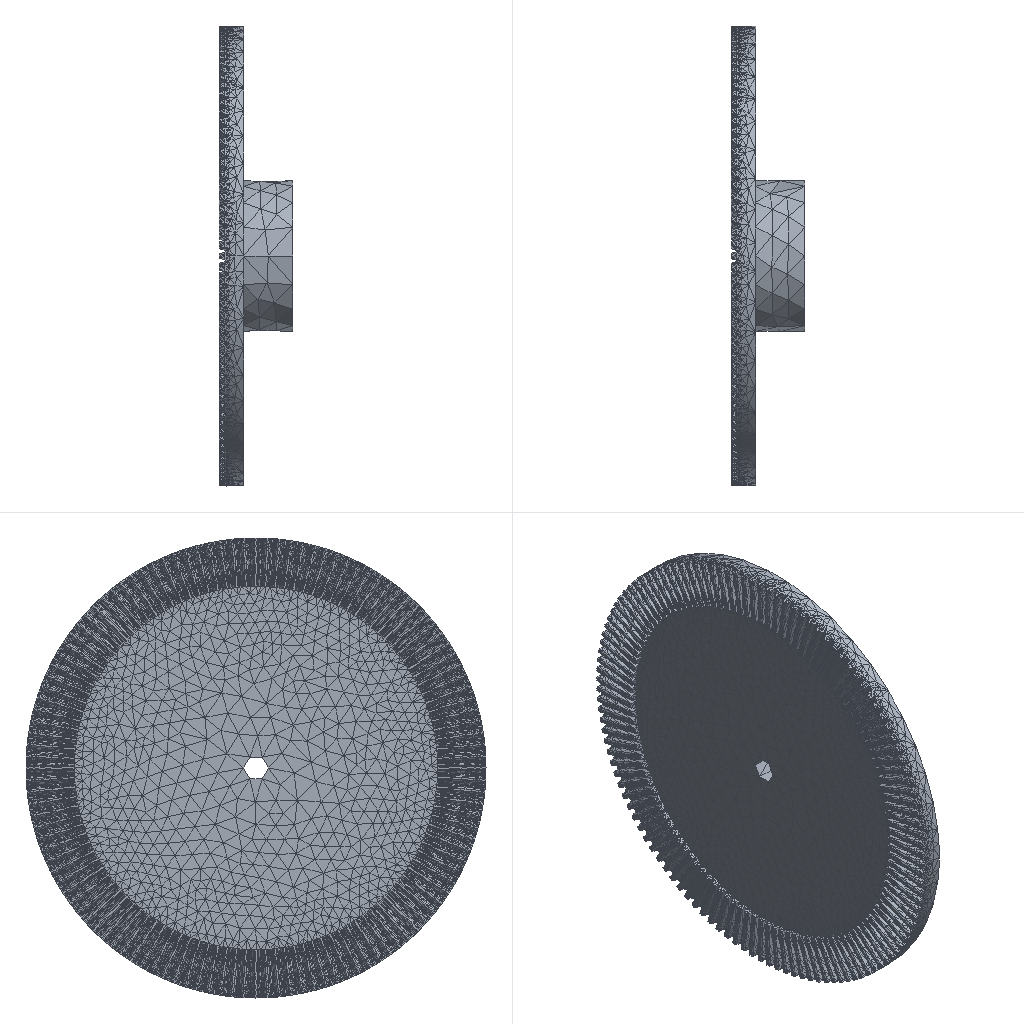Simulation study | ansys workbench
Set-up summary:
category,name,step,type,value,unit,region
solver,ansys_workbench
units,mm-N-s-tonne (MPa),,stated,"/units,MPA"
analysis,LS1,,modal,method=lanb; n_modes=6
load_step,LS1,LS1,modal
mesh,nodes,,,62313
mesh,elements,,,32535
element_type,SOLID187,,,32535
material,45?,,E,200000,tonne s^-2 mm^-1
material,45?,,nu,0.3
material,45?,,density,7.85e-09,tonne mm^-3
material,45?,,conductivity,60.5,tonne mm s^-3 C^-1
material,45?,,specific_heat,4.34e+08,mm^2 s^-2 C^-1
material,45?,,cte,1.2e-05,C^-1
material,45?,,permeability,10000
material,45?,,resistivity,0.00017,ohm mm
bc,Fixed Supports,model,fixed,[dofs=ALL],,_FIXEDSU
named_set,_FIXEDSU,,node,68
Ansys APDL input file, long lists of numbers shortened:
/batch
/config,noeldb,1     ! force off writing results to database
*get,_wallstrt,active,,time,wall
! ANSYS input file written by Workbench version 2022 R1
! File used for geometry attach:
/title,wbnew--__ (B5)
! ****** Begin Custom Load Command Snippet ******
/COM, ACT Extensions:
/COM,     LSDYNA, 2021.1
/COM,
! ****** End   Custom Load Command Snippet ******
*DIM,_wb_ProjectScratch_dir,string,248
_wb_ProjectScratch_dir(1) = ''
*DIM,_wb_SolverFiles_dir,string,248
_wb_SolverFiles_dir(1) = ''
*DIM,_wb_userfiles_dir,string,248
_wb_userfiles_dir(1) = ''
/com,--- Data in consistent NMM units. See Solving Units in the help system for more information.
/units,MPA
/nopr
/wb,file,start              !  signify a WB generated input file
/prep7
! Turn off shape checking because checks already performed inside WB mesher.
! See help system for more information.
SHPP,OFF,,NOWARN
/nolist
etcon,set             ! allow ANSYS to choose best KEYOP's for 180x elements, resets any applicable keyopt to MAPDL defaults
/com,*********** Nodes for the whole assembly ***********
nblock,3,,68544
(1i9,3e20.9e3)
        1    -1.600000000E+01     2.450000000E+01     0.000000000E+00
! (62312 more lines like these left out)
-1
/wb,elem,start            !  set before creation of elements
/com,*********** Elements for Body 1 "60-FreeParts|__-__1" ***********
et,1,187
eblock,19,solid,,32535
(19i9)
        1        1        1        1        0        0        0        0       10        0        1     6731    10302     6958     7188    51539    53095    51534    51537
! (65069 more lines like these left out)
-1
/wb,elem,end               !  done creating elements
/com,*********** Send User Defined Coordinate System(s) ***********
csys,0
toffst,273.15,  ! Temperature offset from absolute zero
/com,*********** Set Reference Temperature ***********
tref,22.
/wb,mat,start              !  starting to send materials
/com,*********** Send Materials ***********
Temperature = 'TEMP' ! Temperature
MP,DENS,1,7.85e-09,	! tonne mm^-3
MP,ALPX,1,1.2e-05,	! C^-1
MP,C,1,434000000,	! mm^2 s^-2 C^-1
MP,KXX,1,60.5,	! tonne mm s^-3 C^-1
MP,RSVX,1,0.00017,	! ohm mm
MP,EX,1,200000,	! tonne s^-2 mm^-1
MP,NUXY,1,0.3,
MP,MURX,1,10000,
/wb,mat,end                !  done sending materials
!************************* Model Summary ********************
!60-FreeParts|__-__1,	45钢,	matid,	1
!************************* End Model Summary ********************
! get the diagonal of the bounding box. Needed later for other things
*get,_xmin,node,,mnloc,x
*get,_ymin,node,,mnloc,y
*get,_zmin,node,,mnloc,z
*get,_xmax,node,,mxloc,x
*get,_ymax,node,,mxloc,y
*get,_zmax,node,,mxloc,z
_ASMDIAG=(_xmax-_xmin)*(_xmax-_xmin)+(_ymax-_ymin)*(_ymax-_ymin)+(_zmax-_zmin)*(_zmax-_zmin)
_ASMDIAG=SQRT(_ASMDIAG)
/wb,contact,start          !  starting to send contact
/wb,contact,end            !  done creating contacts
/golist
/wb,load,start             !  starting to send loads
/com,*********** Fixed Supports ***********
CMBLOCK,_FIXEDSU,NODE,       68
(8i10)
       407       408       409       410       411       412       413       414
! (8 more lines like these left out)
cmsel,s,_FIXEDSU
d,all,all
nsel,all
/gst,on,on
fini
*get,_numnode,node,0,count
*get,_numelem,elem,0,count
*get, _MAXELEMNUM, elem, 0, NUM, MAX
*get, _MAXNODENUM, node, 0, NUM, MAX
*get, _MAXELEMTYPE, etyp, 0, NUM, MAX
*get, _MAXREALCONST, real, 0, NUM, MAX
/go
/wb,load,end               !  done creating loads
/com,--- Number of total nodes = %_numnode%
/com,--- Number of contact elements = 0
/com,--- Number of spring elements = 0
/com,--- Number of bearing elements = 0
/com,--- Number of solid elements = 32535
/com,--- Number of condensed parts = 0
/com,--- Number of total elements = %_numelem%
*get,_wallbsol,active,,time,wall
/solu
antype,2                   ! modal analysis
_thickRatio=  1     ! Ratio of thick parts in the model
modopt,lanb,6
outres,erase
outres,all,none
outres,nsol,all
outres,etmp,all
mxpand                    ! default expand in case of complex solution
dmpopt,esav,no
dmpopt,emat,no
dmpopt,full,no
! *********** WB SOLVE COMMAND ***********
! check interactive state
*get,ANSINTER_,active,,int
*if,ANSINTER_,ne,0,then
/eof
*endif
solve
/com *************** Write FE CONNECTORS *********
CEWRITE,file,ce,,INTE
*get,_nmodalsolproc,active,0,numcpu
fini
/nopr
*get,_numnode,node,0,count
*get,_numelem,elem,0,count
*get, _MAXELEMNUM, elem, 0, NUM, MAX
*get, _MAXNODENUM, node, 0, NUM, MAX,,,INTERNAL
*get, _MAXELEMTYPE, etyp, 0, NUM, MAX
*get, _MAXREALCONST, real, 0, NUM, MAX
/gopr
*get,_wallasol,active,,time,wall
/post1
/nopr
*dim,_direction,CHAR,6,1
_direction(1) = 'X'
_direction(2) = 'Y'
_direction(3) = 'Z'
_direction(4) = 'ROTX'
_direction(5) = 'ROTY'
_direction(6) = 'ROTZ'
*get,_lastLS,active,0,set,LSTP
*get,_beginset,active,0,set,nset,first,_lastLS
*get,_endset,active,0,set,nset,last,_lastLS
_nummodes = 0
*if,_endset,gt,0,then
_nummodes = _endset - _beginset + 1
*endif
*do,i_mode,1,_nummodes
   *do,j_component,1,6
			*get,PFACT_%i_mode%_%j_component%,MODE,%i_mode%,PFACT,,DIREC,_direction(%j_component%)
   *enddo
*enddo
*dim,_tmdirection,CHAR,6,1
_tmdirection(1) = 'X'
_tmdirection(2) = 'Y'
_tmdirection(3) = 'Z'
_tmdirection(4) = 'X'
_tmdirection(5) = 'Y'
_tmdirection(6) = 'Z'
*do,j_component,1,6
    *if,j_component,gt,3,then
        *get,TOTALMASS_%j_component%,ELEM,0,IOR,_tmdirection(%j_component%)
    *else
        *get,TOTALMASS_%j_component%,ELEM,0,MTOT,_tmdirection(%j_component%)
    *endif
*enddo
/gopr
xmlo,ENCODING,ISO-8859-1
xmlo,parm
/xml,parm,xml
fini
/gopr
*get,_walldone,active,,time,wall
_preptime=(_wallbsol-_wallstrt)*3600
_solvtime=(_wallasol-_wallbsol)*3600
_posttime=(_walldone-_wallasol)*3600
_totaltim=(_walldone-_wallstrt)*3600
*get,_dlbratio,active,0,solu,dlbr
*get,_combtime,active,0,solu,comb
*get,_ssmode,active,0,solu,ssmm
*get,_ndofs,active,0,solu,ndof
/fclean				!clean distributed files
/com,--- Total number of nodes = %_numnode%
/com,--- Total number of elements = %_numelem%
/com,--- Element load balance ratio = %_dlbratio%
/com,--- Time to combine distributed files = %_combtime%
/com,--- Sparse memory mode = %_ssmode%
/com,--- Number of DOF = %_ndofs%
/wb,file,end               ! done with WB generated input
Results summary:
result,analyses[0].index,,,1
result,analyses[0].system,,,SYS
result,analyses[0].deck,,,deck.dat
result,analyses[0].solve_status,,,completed
result,analyses[0].analysis_type,,,modal
result,analyses[0].physics,,,mechanical
result,analyses[0].unit_system,,,"NMM: mm, ton, N, s, mV, mA, degC"
result,analyses[0].n_sets,,,6
result,analyses[0].modal_frequencies_hz[1],,,1386.53
result,analyses[0].modal_frequencies_hz[2],,,1389.04
result,analyses[0].modal_frequencies_hz[3],,,1496.37
result,analyses[0].modal_frequencies_hz[4],,,1761.95
result,analyses[0].modal_frequencies_hz[5],,,1764.17
result,analyses[0].modal_frequencies_hz[6],,,1851.44